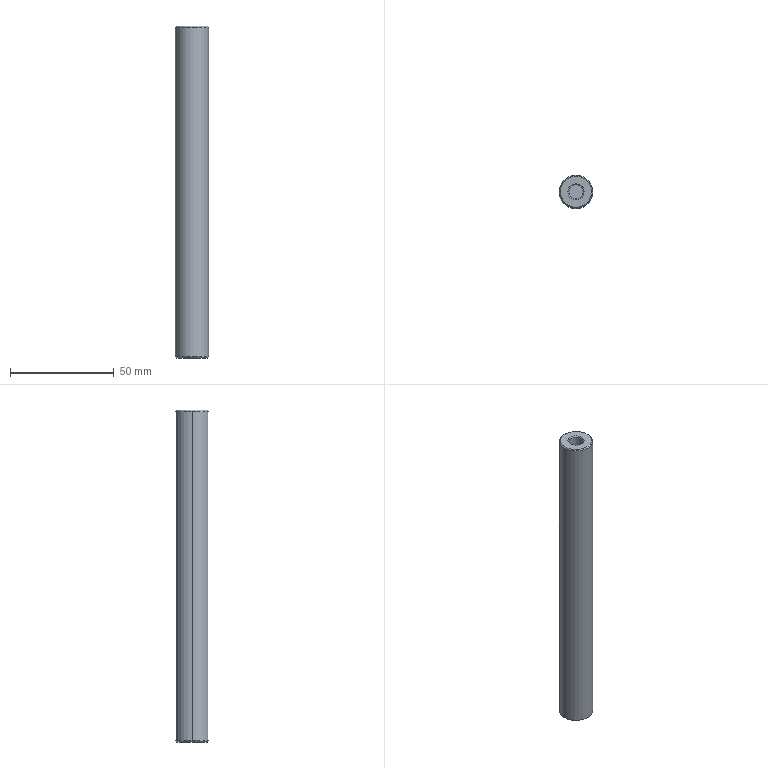Part | STEP file | Column | 1 solid | 18 faces | box 16 x 16 x 160 mm | volume 30717 mm3 | cone 8 | cylinder 6 | plane 4 | commonest cylinder face diameters 6.8 x4 16 x2
STEP:
#1=CARTESIAN_POINT('',(0.,0.,0.));
#2=DIRECTION('',(0.,0.,1.));
#3=DIRECTION('',(1.,0.,0.));
#4=AXIS2_PLACEMENT_3D('',#1,#2,#3);
#5=CARTESIAN_POINT('',(-8.,0.,159.5));
#6=VERTEX_POINT('',#5);
#7=CARTESIAN_POINT('',(8.,0.,159.5));
#8=VERTEX_POINT('',#7);
#9=CARTESIAN_POINT('',(0.,0.,159.5));
#10=DIRECTION('',(0.,0.,-1.));
#11=DIRECTION('',(-1.,0.,0.));
#12=AXIS2_PLACEMENT_3D('',#9,#10,#11);
#13=CIRCLE('',#12,8.);
#14=CARTESIAN_POINT('',(0.,0.,160.));
#15=DIRECTION('',(0.,0.,-1.));
#16=DIRECTION('',(-1.,0.,0.));
#17=AXIS2_PLACEMENT_3D('',#14,#15,#16);
#18=CYLINDRICAL_SURFACE('',#17,8.);
#19=CARTESIAN_POINT('',(0.,0.5));
#20=DIRECTION('',(1.,0.));
#21=VECTOR('',#20,1.);
#22=LINE('',#19,#21);
#23=(GEOMETRIC_REPRESENTATION_CONTEXT(2)PARAMETRIC_REPRESENTATION_CONTEXT()REPRESENTATION_CONTEXT('',''));
#24=DEFINITIONAL_REPRESENTATION('',(#22),#23);
#25=PCURVE('',#18,#24);
#26=CARTESIAN_POINT('',(0.,0.,159.5));
#27=DIRECTION('',(0.,0.,-1.));
#28=DIRECTION('',(-1.,0.,0.));
#29=AXIS2_PLACEMENT_3D('',#26,#27,#28);
#30=CONICAL_SURFACE('',#29,8.,0.7854);
#31=CARTESIAN_POINT('',(0.,0.));
#32=DIRECTION('',(1.,0.));
#33=VECTOR('',#32,1.);
#34=LINE('',#31,#33);
#35=(GEOMETRIC_REPRESENTATION_CONTEXT(2)PARAMETRIC_REPRESENTATION_CONTEXT()REPRESENTATION_CONTEXT('',''));
#36=DEFINITIONAL_REPRESENTATION('',(#34),#35);
#37=PCURVE('',#30,#36);
#38=SURFACE_CURVE('',#13,(#25,#37),.PCURVE_S1.);
#39=EDGE_CURVE('',#6,#8,#38,.T.);
#40=ORIENTED_EDGE('',*,*,#39,.T.);
#41=CARTESIAN_POINT('',(8.,0.,0.5));
#42=VERTEX_POINT('',#41);
#43=CARTESIAN_POINT('',(8.,0.,160.));
#44=DIRECTION('',(0.,0.,-1.));
#45=VECTOR('',#44,1.);
#46=LINE('',#43,#45);
#47=CARTESIAN_POINT('',(3.142,0.));
#48=DIRECTION('',(0.,1.));
#49=VECTOR('',#48,1.);
#50=LINE('',#47,#49);
#51=(GEOMETRIC_REPRESENTATION_CONTEXT(2)PARAMETRIC_REPRESENTATION_CONTEXT()REPRESENTATION_CONTEXT('',''));
#52=DEFINITIONAL_REPRESENTATION('',(#50),#51);
#53=PCURVE('',#18,#52);
#54=CARTESIAN_POINT('',(0.,0.,160.));
#55=DIRECTION('',(0.,0.,-1.));
#56=DIRECTION('',(-1.,0.,0.));
#57=AXIS2_PLACEMENT_3D('',#54,#55,#56);
#58=CYLINDRICAL_SURFACE('',#57,8.);
#59=CARTESIAN_POINT('',(3.142,0.));
#60=DIRECTION('',(0.,1.));
#61=VECTOR('',#60,1.);
#62=LINE('',#59,#61);
#63=(GEOMETRIC_REPRESENTATION_CONTEXT(2)PARAMETRIC_REPRESENTATION_CONTEXT()REPRESENTATION_CONTEXT('',''));
#64=DEFINITIONAL_REPRESENTATION('',(#62),#63);
#65=PCURVE('',#58,#64);
#66=SURFACE_CURVE('',#46,(#53,#65),.PCURVE_S1.);
#67=EDGE_CURVE('',#8,#42,#66,.T.);
#68=ORIENTED_EDGE('',*,*,#67,.T.);
#69=CARTESIAN_POINT('',(-8.,0.,0.5));
#70=VERTEX_POINT('',#69);
#71=CARTESIAN_POINT('',(0.,0.,0.5));
#72=DIRECTION('',(0.,0.,1.));
#73=DIRECTION('',(-1.,0.,0.));
#74=AXIS2_PLACEMENT_3D('',#71,#72,#73);
#75=CIRCLE('',#74,8.);
#76=CARTESIAN_POINT('',(6.283,159.5));
#77=DIRECTION('',(-1.,0.));
#78=VECTOR('',#77,1.);
#79=LINE('',#76,#78);
#80=(GEOMETRIC_REPRESENTATION_CONTEXT(2)PARAMETRIC_REPRESENTATION_CONTEXT()REPRESENTATION_CONTEXT('',''));
#81=DEFINITIONAL_REPRESENTATION('',(#79),#80);
#82=PCURVE('',#18,#81);
#83=CARTESIAN_POINT('',(0.,0.,0.5));
#84=DIRECTION('',(0.,0.,1.));
#85=DIRECTION('',(1.,0.,0.));
#86=AXIS2_PLACEMENT_3D('',#83,#84,#85);
#87=CONICAL_SURFACE('',#86,8.,0.7854);
#88=CARTESIAN_POINT('',(-3.142,0.));
#89=DIRECTION('',(1.,0.));
#90=VECTOR('',#89,1.);
#91=LINE('',#88,#90);
#92=(GEOMETRIC_REPRESENTATION_CONTEXT(2)PARAMETRIC_REPRESENTATION_CONTEXT()REPRESENTATION_CONTEXT('',''));
#93=DEFINITIONAL_REPRESENTATION('',(#91),#92);
#94=PCURVE('',#87,#93);
#95=SURFACE_CURVE('',#75,(#82,#94),.PCURVE_S1.);
#96=EDGE_CURVE('',#42,#70,#95,.T.);
#97=ORIENTED_EDGE('',*,*,#96,.T.);
#98=CARTESIAN_POINT('',(-8.,0.,160.));
#99=DIRECTION('',(0.,0.,-1.));
#100=VECTOR('',#99,1.);
#101=LINE('',#98,#100);
#102=CARTESIAN_POINT('',(0.,0.));
#103=DIRECTION('',(0.,1.));
#104=VECTOR('',#103,1.);
#105=LINE('',#102,#104);
#106=(GEOMETRIC_REPRESENTATION_CONTEXT(2)PARAMETRIC_REPRESENTATION_CONTEXT()REPRESENTATION_CONTEXT('',''));
#107=DEFINITIONAL_REPRESENTATION('',(#105),#106);
#108=PCURVE('',#18,#107);
#109=CARTESIAN_POINT('',(6.283,0.));
#110=DIRECTION('',(0.,1.));
#111=VECTOR('',#110,1.);
#112=LINE('',#109,#111);
#113=(GEOMETRIC_REPRESENTATION_CONTEXT(2)PARAMETRIC_REPRESENTATION_CONTEXT()REPRESENTATION_CONTEXT('',''));
#114=DEFINITIONAL_REPRESENTATION('',(#112),#113);
#115=PCURVE('',#58,#114);
#116=SURFACE_CURVE('',#101,(#108,#115),.PCURVE_S1.);
#117=EDGE_CURVE('',#6,#70,#116,.T.);
#118=ORIENTED_EDGE('',*,*,#117,.F.);
#119=EDGE_LOOP('',(#40,#68,#97,#118));
#120=FACE_BOUND('',#119,.T.);
#121=ADVANCED_FACE('',(#120),#18,.T.);
#122=CARTESIAN_POINT('',(7.5,0.,0.));
#123=VERTEX_POINT('',#122);
#124=CARTESIAN_POINT('',(-7.5,0.,0.));
#125=VERTEX_POINT('',#124);
#126=CARTESIAN_POINT('',(0.,0.,0.));
#127=DIRECTION('',(0.,0.,1.));
#128=DIRECTION('',(1.,0.,0.));
#129=AXIS2_PLACEMENT_3D('',#126,#127,#128);
#130=CIRCLE('',#129,7.5);
#131=CARTESIAN_POINT('',(0.,-0.5));
#132=DIRECTION('',(1.,0.));
#133=VECTOR('',#132,1.);
#134=LINE('',#131,#133);
#135=(GEOMETRIC_REPRESENTATION_CONTEXT(2)PARAMETRIC_REPRESENTATION_CONTEXT()REPRESENTATION_CONTEXT('',''));
#136=DEFINITIONAL_REPRESENTATION('',(#134),#135);
#137=PCURVE('',#87,#136);
#138=CARTESIAN_POINT('',(0.,0.,0.));
#139=DIRECTION('',(0.,0.,1.));
#140=DIRECTION('',(1.,0.,0.));
#141=AXIS2_PLACEMENT_3D('',#138,#139,#140);
#142=PLANE('',#141);
#143=CARTESIAN_POINT('',(0.,0.));
#144=DIRECTION('',(1.,0.));
#145=AXIS2_PLACEMENT_2D('',#143,#144);
#146=CIRCLE('',#145,7.5);
#147=(GEOMETRIC_REPRESENTATION_CONTEXT(2)PARAMETRIC_REPRESENTATION_CONTEXT()REPRESENTATION_CONTEXT('',''));
#148=DEFINITIONAL_REPRESENTATION('',(#146),#147);
#149=PCURVE('',#142,#148);
#150=SURFACE_CURVE('',#130,(#137,#149),.PCURVE_S1.);
#151=EDGE_CURVE('',#123,#125,#150,.T.);
#152=ORIENTED_EDGE('',*,*,#151,.T.);
#153=CARTESIAN_POINT('',(-8.,0.,0.5));
#154=DIRECTION('',(-0.7071,0.,0.7071));
#155=VECTOR('',#154,1.);
#156=LINE('',#153,#155);
#157=CARTESIAN_POINT('',(3.142,0.));
#158=DIRECTION('',(0.,1.));
#159=VECTOR('',#158,1.);
#160=LINE('',#157,#159);
#161=(GEOMETRIC_REPRESENTATION_CONTEXT(2)PARAMETRIC_REPRESENTATION_CONTEXT()REPRESENTATION_CONTEXT('',''));
#162=DEFINITIONAL_REPRESENTATION('',(#160),#161);
#163=PCURVE('',#87,#162);
#164=CARTESIAN_POINT('',(0.,0.,0.5));
#165=DIRECTION('',(0.,0.,1.));
#166=DIRECTION('',(1.,0.,0.));
#167=AXIS2_PLACEMENT_3D('',#164,#165,#166);
#168=CONICAL_SURFACE('',#167,8.,0.7854);
#169=CARTESIAN_POINT('',(3.142,0.));
#170=DIRECTION('',(0.,1.));
#171=VECTOR('',#170,1.);
#172=LINE('',#169,#171);
#173=(GEOMETRIC_REPRESENTATION_CONTEXT(2)PARAMETRIC_REPRESENTATION_CONTEXT()REPRESENTATION_CONTEXT('',''));
#174=DEFINITIONAL_REPRESENTATION('',(#172),#173);
#175=PCURVE('',#168,#174);
#176=SURFACE_CURVE('',#156,(#163,#175),.PCURVE_S1.);
#177=EDGE_CURVE('',#125,#70,#176,.T.);
#178=ORIENTED_EDGE('',*,*,#177,.T.);
#179=ORIENTED_EDGE('',*,*,#96,.F.);
#180=CARTESIAN_POINT('',(8.,0.,0.5));
#181=DIRECTION('',(0.7071,0.,0.7071));
#182=VECTOR('',#181,1.);
#183=LINE('',#180,#182);
#184=CARTESIAN_POINT('',(0.,0.));
#185=DIRECTION('',(0.,1.));
#186=VECTOR('',#185,1.);
#187=LINE('',#184,#186);
#188=(GEOMETRIC_REPRESENTATION_CONTEXT(2)PARAMETRIC_REPRESENTATION_CONTEXT()REPRESENTATION_CONTEXT('',''));
#189=DEFINITIONAL_REPRESENTATION('',(#187),#188);
#190=PCURVE('',#87,#189);
#191=CARTESIAN_POINT('',(6.283,0.));
#192=DIRECTION('',(0.,1.));
#193=VECTOR('',#192,1.);
#194=LINE('',#191,#193);
#195=(GEOMETRIC_REPRESENTATION_CONTEXT(2)PARAMETRIC_REPRESENTATION_CONTEXT()REPRESENTATION_CONTEXT('',''));
#196=DEFINITIONAL_REPRESENTATION('',(#194),#195);
#197=PCURVE('',#168,#196);
#198=SURFACE_CURVE('',#183,(#190,#197),.PCURVE_S1.);
#199=EDGE_CURVE('',#123,#42,#198,.T.);
#200=ORIENTED_EDGE('',*,*,#199,.F.);
#201=EDGE_LOOP('',(#152,#178,#179,#200));
#202=FACE_BOUND('',#201,.T.);
#203=ADVANCED_FACE('',(#202),#87,.T.);
#204=CARTESIAN_POINT('',(-7.5,0.,160.));
#205=VERTEX_POINT('',#204);
#206=CARTESIAN_POINT('',(7.5,0.,160.));
#207=VERTEX_POINT('',#206);
#208=CARTESIAN_POINT('',(0.,0.,160.));
#209=DIRECTION('',(0.,0.,-1.));
#210=DIRECTION('',(-1.,0.,0.));
#211=AXIS2_PLACEMENT_3D('',#208,#209,#210);
#212=CIRCLE('',#211,7.5);
#213=CARTESIAN_POINT('',(0.,-0.5));
#214=DIRECTION('',(1.,0.));
#215=VECTOR('',#214,1.);
#216=LINE('',#213,#215);
#217=(GEOMETRIC_REPRESENTATION_CONTEXT(2)PARAMETRIC_REPRESENTATION_CONTEXT()REPRESENTATION_CONTEXT('',''));
#218=DEFINITIONAL_REPRESENTATION('',(#216),#217);
#219=PCURVE('',#30,#218);
#220=CARTESIAN_POINT('',(0.,0.,160.));
#221=DIRECTION('',(0.,0.,1.));
#222=DIRECTION('',(1.,0.,0.));
#223=AXIS2_PLACEMENT_3D('',#220,#221,#222);
#224=PLANE('',#223);
#225=CARTESIAN_POINT('',(-7.5,0.));
#226=CARTESIAN_POINT('',(-7.5,12.99));
#227=CARTESIAN_POINT('',(3.75,6.495));
#228=CARTESIAN_POINT('',(15.,0.));
#229=CARTESIAN_POINT('',(3.75,-6.495));
#230=CARTESIAN_POINT('',(-7.5,-12.99));
#231=CARTESIAN_POINT('',(-7.5,0.));
#232=(BOUNDED_CURVE()B_SPLINE_CURVE(2,(#225,#226,#227,#228,#229,#230,#231),.UNSPECIFIED.,.T.,.F.)B_SPLINE_CURVE_WITH_KNOTS((1,2,2,2,2,1),(-2.094,0.,2.094,4.189,6.283,8.378),.UNSPECIFIED.)CURVE()GEOMETRIC_REPRESENTATION_ITEM()RATIONAL_B_SPLINE_CURVE((1.,0.5,1.,0.5,1.,0.5,1.))REPRESENTATION_ITEM(''));
#233=(GEOMETRIC_REPRESENTATION_CONTEXT(2)PARAMETRIC_REPRESENTATION_CONTEXT()REPRESENTATION_CONTEXT('',''));
#234=DEFINITIONAL_REPRESENTATION('',(#232),#233);
#235=PCURVE('',#224,#234);
#236=SURFACE_CURVE('',#212,(#219,#235),.PCURVE_S1.);
#237=EDGE_CURVE('',#205,#207,#236,.T.);
#238=ORIENTED_EDGE('',*,*,#237,.T.);
#239=CARTESIAN_POINT('',(8.,0.,159.5));
#240=DIRECTION('',(0.7071,0.,-0.7071));
#241=VECTOR('',#240,1.);
#242=LINE('',#239,#241);
#243=CARTESIAN_POINT('',(3.142,0.));
#244=DIRECTION('',(0.,1.));
#245=VECTOR('',#244,1.);
#246=LINE('',#243,#245);
#247=(GEOMETRIC_REPRESENTATION_CONTEXT(2)PARAMETRIC_REPRESENTATION_CONTEXT()REPRESENTATION_CONTEXT('',''));
#248=DEFINITIONAL_REPRESENTATION('',(#246),#247);
#249=PCURVE('',#30,#248);
#250=CARTESIAN_POINT('',(0.,0.,159.5));
#251=DIRECTION('',(0.,0.,-1.));
#252=DIRECTION('',(-1.,0.,0.));
#253=AXIS2_PLACEMENT_3D('',#250,#251,#252);
#254=CONICAL_SURFACE('',#253,8.,0.7854);
#255=CARTESIAN_POINT('',(3.142,0.));
#256=DIRECTION('',(0.,1.));
#257=VECTOR('',#256,1.);
#258=LINE('',#255,#257);
#259=(GEOMETRIC_REPRESENTATION_CONTEXT(2)PARAMETRIC_REPRESENTATION_CONTEXT()REPRESENTATION_CONTEXT('',''));
#260=DEFINITIONAL_REPRESENTATION('',(#258),#259);
#261=PCURVE('',#254,#260);
#262=SURFACE_CURVE('',#242,(#249,#261),.PCURVE_S1.);
#263=EDGE_CURVE('',#207,#8,#262,.T.);
#264=ORIENTED_EDGE('',*,*,#263,.T.);
#265=ORIENTED_EDGE('',*,*,#39,.F.);
#266=CARTESIAN_POINT('',(-8.,0.,159.5));
#267=DIRECTION('',(-0.7071,0.,-0.7071));
#268=VECTOR('',#267,1.);
#269=LINE('',#266,#268);
#270=CARTESIAN_POINT('',(0.,0.));
#271=DIRECTION('',(0.,1.));
#272=VECTOR('',#271,1.);
#273=LINE('',#270,#272);
#274=(GEOMETRIC_REPRESENTATION_CONTEXT(2)PARAMETRIC_REPRESENTATION_CONTEXT()REPRESENTATION_CONTEXT('',''));
#275=DEFINITIONAL_REPRESENTATION('',(#273),#274);
#276=PCURVE('',#30,#275);
#277=CARTESIAN_POINT('',(6.283,0.));
#278=DIRECTION('',(0.,1.));
#279=VECTOR('',#278,1.);
#280=LINE('',#277,#279);
#281=(GEOMETRIC_REPRESENTATION_CONTEXT(2)PARAMETRIC_REPRESENTATION_CONTEXT()REPRESENTATION_CONTEXT('',''));
#282=DEFINITIONAL_REPRESENTATION('',(#280),#281);
#283=PCURVE('',#254,#282);
#284=SURFACE_CURVE('',#269,(#276,#283),.PCURVE_S1.);
#285=EDGE_CURVE('',#205,#6,#284,.T.);
#286=ORIENTED_EDGE('',*,*,#285,.F.);
#287=EDGE_LOOP('',(#238,#264,#265,#286));
#288=FACE_BOUND('',#287,.T.);
#289=ADVANCED_FACE('',(#288),#30,.T.);
#290=CARTESIAN_POINT('',(-3.4,0.,0.5));
#291=VERTEX_POINT('',#290);
#292=CARTESIAN_POINT('',(-3.9,0.,0.));
#293=VERTEX_POINT('',#292);
#294=CARTESIAN_POINT('',(-3.9,0.,0.));
#295=DIRECTION('',(-0.7071,0.,-0.7071));
#296=VECTOR('',#295,1.);
#297=LINE('',#294,#296);
#298=CARTESIAN_POINT('',(0.,0.,0.));
#299=DIRECTION('',(0.,0.,-1.));
#300=DIRECTION('',(-1.,0.,0.));
#301=AXIS2_PLACEMENT_3D('',#298,#299,#300);
#302=CONICAL_SURFACE('',#301,3.9,0.7854);
#303=CARTESIAN_POINT('',(6.283,0.));
#304=DIRECTION('',(0.,1.));
#305=VECTOR('',#304,1.);
#306=LINE('',#303,#305);
#307=(GEOMETRIC_REPRESENTATION_CONTEXT(2)PARAMETRIC_REPRESENTATION_CONTEXT()REPRESENTATION_CONTEXT('',''));
#308=DEFINITIONAL_REPRESENTATION('',(#306),#307);
#309=PCURVE('',#302,#308);
#310=CARTESIAN_POINT('',(0.,0.,0.));
#311=DIRECTION('',(0.,0.,-1.));
#312=DIRECTION('',(-1.,0.,0.));
#313=AXIS2_PLACEMENT_3D('',#310,#311,#312);
#314=CONICAL_SURFACE('',#313,3.9,0.7854);
#315=CARTESIAN_POINT('',(0.,0.));
#316=DIRECTION('',(0.,1.));
#317=VECTOR('',#316,1.);
#318=LINE('',#315,#317);
#319=(GEOMETRIC_REPRESENTATION_CONTEXT(2)PARAMETRIC_REPRESENTATION_CONTEXT()REPRESENTATION_CONTEXT('',''));
#320=DEFINITIONAL_REPRESENTATION('',(#318),#319);
#321=PCURVE('',#314,#320);
#322=SURFACE_CURVE('',#297,(#309,#321),.PCURVE_S1.);
#323=EDGE_CURVE('',#291,#293,#322,.T.);
#324=ORIENTED_EDGE('',*,*,#323,.T.);
#325=CARTESIAN_POINT('',(3.9,0.,0.));
#326=VERTEX_POINT('',#325);
#327=CARTESIAN_POINT('',(0.,0.,0.));
#328=DIRECTION('',(0.,0.,-1.));
#329=DIRECTION('',(-1.,0.,0.));
#330=AXIS2_PLACEMENT_3D('',#327,#328,#329);
#331=CIRCLE('',#330,3.9);
#332=CARTESIAN_POINT('',(0.,0.));
#333=DIRECTION('',(1.,0.));
#334=VECTOR('',#333,1.);
#335=LINE('',#332,#334);
#336=(GEOMETRIC_REPRESENTATION_CONTEXT(2)PARAMETRIC_REPRESENTATION_CONTEXT()REPRESENTATION_CONTEXT('',''));
#337=DEFINITIONAL_REPRESENTATION('',(#335),#336);
#338=PCURVE('',#302,#337);
#339=CARTESIAN_POINT('',(-3.9,0.));
#340=CARTESIAN_POINT('',(-3.9,6.755));
#341=CARTESIAN_POINT('',(1.95,3.377));
#342=CARTESIAN_POINT('',(7.8,0.));
#343=CARTESIAN_POINT('',(1.95,-3.377));
#344=CARTESIAN_POINT('',(-3.9,-6.755));
#345=CARTESIAN_POINT('',(-3.9,0.));
#346=(BOUNDED_CURVE()B_SPLINE_CURVE(2,(#339,#340,#341,#342,#343,#344,#345),.UNSPECIFIED.,.T.,.F.)B_SPLINE_CURVE_WITH_KNOTS((1,2,2,2,2,1),(-2.094,0.,2.094,4.189,6.283,8.378),.UNSPECIFIED.)CURVE()GEOMETRIC_REPRESENTATION_ITEM()RATIONAL_B_SPLINE_CURVE((1.,0.5,1.,0.5,1.,0.5,1.))REPRESENTATION_ITEM(''));
#347=(GEOMETRIC_REPRESENTATION_CONTEXT(2)PARAMETRIC_REPRESENTATION_CONTEXT()REPRESENTATION_CONTEXT('',''));
#348=DEFINITIONAL_REPRESENTATION('',(#346),#347);
#349=PCURVE('',#142,#348);
#350=SURFACE_CURVE('',#331,(#338,#349),.PCURVE_S1.);
#351=EDGE_CURVE('',#326,#293,#350,.T.);
#352=ORIENTED_EDGE('',*,*,#351,.F.);
#353=CARTESIAN_POINT('',(3.4,0.,0.5));
#354=VERTEX_POINT('',#353);
#355=CARTESIAN_POINT('',(3.9,0.,0.));
#356=DIRECTION('',(0.7071,0.,-0.7071));
#357=VECTOR('',#356,1.);
#358=LINE('',#355,#357);
#359=CARTESIAN_POINT('',(3.142,0.));
#360=DIRECTION('',(0.,1.));
#361=VECTOR('',#360,1.);
#362=LINE('',#359,#361);
#363=(GEOMETRIC_REPRESENTATION_CONTEXT(2)PARAMETRIC_REPRESENTATION_CONTEXT()REPRESENTATION_CONTEXT('',''));
#364=DEFINITIONAL_REPRESENTATION('',(#362),#363);
#365=PCURVE('',#302,#364);
#366=CARTESIAN_POINT('',(3.142,0.));
#367=DIRECTION('',(0.,1.));
#368=VECTOR('',#367,1.);
#369=LINE('',#366,#368);
#370=(GEOMETRIC_REPRESENTATION_CONTEXT(2)PARAMETRIC_REPRESENTATION_CONTEXT()REPRESENTATION_CONTEXT('',''));
#371=DEFINITIONAL_REPRESENTATION('',(#369),#370);
#372=PCURVE('',#314,#371);
#373=SURFACE_CURVE('',#358,(#365,#372),.PCURVE_S1.);
#374=EDGE_CURVE('',#354,#326,#373,.T.);
#375=ORIENTED_EDGE('',*,*,#374,.F.);
#376=CARTESIAN_POINT('',(0.,0.,0.5));
#377=DIRECTION('',(0.,0.,-1.));
#378=DIRECTION('',(-1.,0.,0.));
#379=AXIS2_PLACEMENT_3D('',#376,#377,#378);
#380=CIRCLE('',#379,3.4);
#381=CARTESIAN_POINT('',(0.,-0.5));
#382=DIRECTION('',(1.,0.));
#383=VECTOR('',#382,1.);
#384=LINE('',#381,#383);
#385=(GEOMETRIC_REPRESENTATION_CONTEXT(2)PARAMETRIC_REPRESENTATION_CONTEXT()REPRESENTATION_CONTEXT('',''));
#386=DEFINITIONAL_REPRESENTATION('',(#384),#385);
#387=PCURVE('',#302,#386);
#388=CARTESIAN_POINT('',(0.,0.,0.));
#389=DIRECTION('',(0.,0.,-1.));
#390=DIRECTION('',(-1.,0.,0.));
#391=AXIS2_PLACEMENT_3D('',#388,#389,#390);
#392=CYLINDRICAL_SURFACE('',#391,3.4);
#393=CARTESIAN_POINT('',(0.,-0.5));
#394=DIRECTION('',(1.,0.));
#395=VECTOR('',#394,1.);
#396=LINE('',#393,#395);
#397=(GEOMETRIC_REPRESENTATION_CONTEXT(2)PARAMETRIC_REPRESENTATION_CONTEXT()REPRESENTATION_CONTEXT('',''));
#398=DEFINITIONAL_REPRESENTATION('',(#396),#397);
#399=PCURVE('',#392,#398);
#400=SURFACE_CURVE('',#380,(#387,#399),.PCURVE_S1.);
#401=EDGE_CURVE('',#354,#291,#400,.T.);
#402=ORIENTED_EDGE('',*,*,#401,.T.);
#403=EDGE_LOOP('',(#324,#352,#375,#402));
#404=FACE_BOUND('',#403,.F.);
#405=ADVANCED_FACE('',(#404),#302,.F.);
#406=CARTESIAN_POINT('',(3.4,0.,159.5));
#407=VERTEX_POINT('',#406);
#408=CARTESIAN_POINT('',(3.9,0.,160.));
#409=VERTEX_POINT('',#408);
#410=CARTESIAN_POINT('',(3.9,0.,160.));
#411=DIRECTION('',(0.7071,0.,0.7071));
#412=VECTOR('',#411,1.);
#413=LINE('',#410,#412);
#414=CARTESIAN_POINT('',(0.,0.,160.));
#415=DIRECTION('',(0.,0.,1.));
#416=DIRECTION('',(1.,0.,0.));
#417=AXIS2_PLACEMENT_3D('',#414,#415,#416);
#418=CONICAL_SURFACE('',#417,3.9,0.7854);
#419=CARTESIAN_POINT('',(6.283,0.));
#420=DIRECTION('',(0.,1.));
#421=VECTOR('',#420,1.);
#422=LINE('',#419,#421);
#423=(GEOMETRIC_REPRESENTATION_CONTEXT(2)PARAMETRIC_REPRESENTATION_CONTEXT()REPRESENTATION_CONTEXT('',''));
#424=DEFINITIONAL_REPRESENTATION('',(#422),#423);
#425=PCURVE('',#418,#424);
#426=CARTESIAN_POINT('',(0.,0.,160.));
#427=DIRECTION('',(0.,0.,1.));
#428=DIRECTION('',(1.,0.,0.));
#429=AXIS2_PLACEMENT_3D('',#426,#427,#428);
#430=CONICAL_SURFACE('',#429,3.9,0.7854);
#431=CARTESIAN_POINT('',(0.,0.));
#432=DIRECTION('',(0.,1.));
#433=VECTOR('',#432,1.);
#434=LINE('',#431,#433);
#435=(GEOMETRIC_REPRESENTATION_CONTEXT(2)PARAMETRIC_REPRESENTATION_CONTEXT()REPRESENTATION_CONTEXT('',''));
#436=DEFINITIONAL_REPRESENTATION('',(#434),#435);
#437=PCURVE('',#430,#436);
#438=SURFACE_CURVE('',#413,(#425,#437),.PCURVE_S1.);
#439=EDGE_CURVE('',#407,#409,#438,.T.);
#440=ORIENTED_EDGE('',*,*,#439,.T.);
#441=CARTESIAN_POINT('',(-3.9,0.,160.));
#442=VERTEX_POINT('',#441);
#443=CARTESIAN_POINT('',(0.,0.,160.));
#444=DIRECTION('',(0.,0.,-1.));
#445=DIRECTION('',(1.,0.,0.));
#446=AXIS2_PLACEMENT_3D('',#443,#444,#445);
#447=CIRCLE('',#446,3.9);
#448=CARTESIAN_POINT('',(6.283,0.));
#449=DIRECTION('',(-1.,0.));
#450=VECTOR('',#449,1.);
#451=LINE('',#448,#450);
#452=(GEOMETRIC_REPRESENTATION_CONTEXT(2)PARAMETRIC_REPRESENTATION_CONTEXT()REPRESENTATION_CONTEXT('',''));
#453=DEFINITIONAL_REPRESENTATION('',(#451),#452);
#454=PCURVE('',#418,#453);
#455=CARTESIAN_POINT('',(3.9,0.));
#456=CARTESIAN_POINT('',(3.9,-6.755));
#457=CARTESIAN_POINT('',(-1.95,-3.377));
#458=CARTESIAN_POINT('',(-7.8,0.));
#459=CARTESIAN_POINT('',(-1.95,3.377));
#460=CARTESIAN_POINT('',(3.9,6.755));
#461=CARTESIAN_POINT('',(3.9,0.));
#462=(BOUNDED_CURVE()B_SPLINE_CURVE(2,(#455,#456,#457,#458,#459,#460,#461),.UNSPECIFIED.,.T.,.F.)B_SPLINE_CURVE_WITH_KNOTS((1,2,2,2,2,1),(-2.094,0.,2.094,4.189,6.283,8.378),.UNSPECIFIED.)CURVE()GEOMETRIC_REPRESENTATION_ITEM()RATIONAL_B_SPLINE_CURVE((1.,0.5,1.,0.5,1.,0.5,1.))REPRESENTATION_ITEM(''));
#463=(GEOMETRIC_REPRESENTATION_CONTEXT(2)PARAMETRIC_REPRESENTATION_CONTEXT()REPRESENTATION_CONTEXT('',''));
#464=DEFINITIONAL_REPRESENTATION('',(#462),#463);
#465=PCURVE('',#224,#464);
#466=SURFACE_CURVE('',#447,(#454,#465),.PCURVE_S1.);
#467=EDGE_CURVE('',#409,#442,#466,.T.);
#468=ORIENTED_EDGE('',*,*,#467,.T.);
#469=CARTESIAN_POINT('',(-3.4,0.,159.5));
#470=VERTEX_POINT('',#469);
#471=CARTESIAN_POINT('',(-3.9,0.,160.));
#472=DIRECTION('',(-0.7071,0.,0.7071));
#473=VECTOR('',#472,1.);
#474=LINE('',#471,#473);
#475=CARTESIAN_POINT('',(3.142,0.));
#476=DIRECTION('',(0.,1.));
#477=VECTOR('',#476,1.);
#478=LINE('',#475,#477);
#479=(GEOMETRIC_REPRESENTATION_CONTEXT(2)PARAMETRIC_REPRESENTATION_CONTEXT()REPRESENTATION_CONTEXT('',''));
#480=DEFINITIONAL_REPRESENTATION('',(#478),#479);
#481=PCURVE('',#418,#480);
#482=CARTESIAN_POINT('',(3.142,0.));
#483=DIRECTION('',(0.,1.));
#484=VECTOR('',#483,1.);
#485=LINE('',#482,#484);
#486=(GEOMETRIC_REPRESENTATION_CONTEXT(2)PARAMETRIC_REPRESENTATION_CONTEXT()REPRESENTATION_CONTEXT('',''));
#487=DEFINITIONAL_REPRESENTATION('',(#485),#486);
#488=PCURVE('',#430,#487);
#489=SURFACE_CURVE('',#474,(#481,#488),.PCURVE_S1.);
#490=EDGE_CURVE('',#470,#442,#489,.T.);
#491=ORIENTED_EDGE('',*,*,#490,.F.);
#492=CARTESIAN_POINT('',(0.,0.,159.5));
#493=DIRECTION('',(0.,0.,1.));
#494=DIRECTION('',(1.,0.,0.));
#495=AXIS2_PLACEMENT_3D('',#492,#493,#494);
#496=CIRCLE('',#495,3.4);
#497=CARTESIAN_POINT('',(0.,-0.5));
#498=DIRECTION('',(1.,0.));
#499=VECTOR('',#498,1.);
#500=LINE('',#497,#499);
#501=(GEOMETRIC_REPRESENTATION_CONTEXT(2)PARAMETRIC_REPRESENTATION_CONTEXT()REPRESENTATION_CONTEXT('',''));
#502=DEFINITIONAL_REPRESENTATION('',(#500),#501);
#503=PCURVE('',#418,#502);
#504=CARTESIAN_POINT('',(0.,0.,160.));
#505=DIRECTION('',(0.,0.,1.));
#506=DIRECTION('',(1.,0.,0.));
#507=AXIS2_PLACEMENT_3D('',#504,#505,#506);
#508=CYLINDRICAL_SURFACE('',#507,3.4);
#509=CARTESIAN_POINT('',(0.,-0.5));
#510=DIRECTION('',(1.,0.));
#511=VECTOR('',#510,1.);
#512=LINE('',#509,#511);
#513=(GEOMETRIC_REPRESENTATION_CONTEXT(2)PARAMETRIC_REPRESENTATION_CONTEXT()REPRESENTATION_CONTEXT('',''));
#514=DEFINITIONAL_REPRESENTATION('',(#512),#513);
#515=PCURVE('',#508,#514);
#516=SURFACE_CURVE('',#496,(#503,#515),.PCURVE_S1.);
#517=EDGE_CURVE('',#470,#407,#516,.T.);
#518=ORIENTED_EDGE('',*,*,#517,.T.);
#519=EDGE_LOOP('',(#440,#468,#491,#518));
#520=FACE_BOUND('',#519,.F.);
#521=ADVANCED_FACE('',(#520),#418,.F.);
#522=CARTESIAN_POINT('',(-3.4,0.,19.75));
#523=VERTEX_POINT('',#522);
#524=CARTESIAN_POINT('',(-3.4,0.,0.));
#525=DIRECTION('',(0.,0.,-1.));
#526=VECTOR('',#525,1.);
#527=LINE('',#524,#526);
#528=CARTESIAN_POINT('',(6.283,0.));
#529=DIRECTION('',(0.,1.));
#530=VECTOR('',#529,1.);
#531=LINE('',#528,#530);
#532=(GEOMETRIC_REPRESENTATION_CONTEXT(2)PARAMETRIC_REPRESENTATION_CONTEXT()REPRESENTATION_CONTEXT('',''));
#533=DEFINITIONAL_REPRESENTATION('',(#531),#532);
#534=PCURVE('',#392,#533);
#535=CARTESIAN_POINT('',(0.,0.,0.));
#536=DIRECTION('',(0.,0.,-1.));
#537=DIRECTION('',(-1.,0.,0.));
#538=AXIS2_PLACEMENT_3D('',#535,#536,#537);
#539=CYLINDRICAL_SURFACE('',#538,3.4);
#540=CARTESIAN_POINT('',(0.,0.));
#541=DIRECTION('',(0.,1.));
#542=VECTOR('',#541,1.);
#543=LINE('',#540,#542);
#544=(GEOMETRIC_REPRESENTATION_CONTEXT(2)PARAMETRIC_REPRESENTATION_CONTEXT()REPRESENTATION_CONTEXT('',''));
#545=DEFINITIONAL_REPRESENTATION('',(#543),#544);
#546=PCURVE('',#539,#545);
#547=SURFACE_CURVE('',#527,(#534,#546),.PCURVE_S1.);
#548=EDGE_CURVE('',#523,#291,#547,.T.);
#549=ORIENTED_EDGE('',*,*,#548,.T.);
#550=ORIENTED_EDGE('',*,*,#401,.F.);
#551=CARTESIAN_POINT('',(3.4,0.,19.75));
#552=VERTEX_POINT('',#551);
#553=CARTESIAN_POINT('',(3.4,0.,0.));
#554=DIRECTION('',(0.,0.,-1.));
#555=VECTOR('',#554,1.);
#556=LINE('',#553,#555);
#557=CARTESIAN_POINT('',(3.142,0.));
#558=DIRECTION('',(0.,1.));
#559=VECTOR('',#558,1.);
#560=LINE('',#557,#559);
#561=(GEOMETRIC_REPRESENTATION_CONTEXT(2)PARAMETRIC_REPRESENTATION_CONTEXT()REPRESENTATION_CONTEXT('',''));
#562=DEFINITIONAL_REPRESENTATION('',(#560),#561);
#563=PCURVE('',#392,#562);
#564=CARTESIAN_POINT('',(3.142,0.));
#565=DIRECTION('',(0.,1.));
#566=VECTOR('',#565,1.);
#567=LINE('',#564,#566);
#568=(GEOMETRIC_REPRESENTATION_CONTEXT(2)PARAMETRIC_REPRESENTATION_CONTEXT()REPRESENTATION_CONTEXT('',''));
#569=DEFINITIONAL_REPRESENTATION('',(#567),#568);
#570=PCURVE('',#539,#569);
#571=SURFACE_CURVE('',#556,(#563,#570),.PCURVE_S1.);
#572=EDGE_CURVE('',#552,#354,#571,.T.);
#573=ORIENTED_EDGE('',*,*,#572,.F.);
#574=CARTESIAN_POINT('',(0.,0.,19.75));
#575=DIRECTION('',(0.,0.,-1.));
#576=DIRECTION('',(-1.,0.,0.));
#577=AXIS2_PLACEMENT_3D('',#574,#575,#576);
#578=CIRCLE('',#577,3.4);
#579=CARTESIAN_POINT('',(0.,-19.75));
#580=DIRECTION('',(1.,0.));
#581=VECTOR('',#580,1.);
#582=LINE('',#579,#581);
#583=(GEOMETRIC_REPRESENTATION_CONTEXT(2)PARAMETRIC_REPRESENTATION_CONTEXT()REPRESENTATION_CONTEXT('',''));
#584=DEFINITIONAL_REPRESENTATION('',(#582),#583);
#585=PCURVE('',#392,#584);
#586=CARTESIAN_POINT('',(0.,0.,19.75));
#587=DIRECTION('',(0.,0.,1.));
#588=DIRECTION('',(1.,0.,0.));
#589=AXIS2_PLACEMENT_3D('',#586,#587,#588);
#590=PLANE('',#589);
#591=CARTESIAN_POINT('',(-3.4,0.));
#592=CARTESIAN_POINT('',(-3.4,5.889));
#593=CARTESIAN_POINT('',(1.7,2.944));
#594=CARTESIAN_POINT('',(6.8,0.));
#595=CARTESIAN_POINT('',(1.7,-2.944));
#596=CARTESIAN_POINT('',(-3.4,-5.889));
#597=CARTESIAN_POINT('',(-3.4,0.));
#598=(BOUNDED_CURVE()B_SPLINE_CURVE(2,(#591,#592,#593,#594,#595,#596,#597),.UNSPECIFIED.,.T.,.F.)B_SPLINE_CURVE_WITH_KNOTS((1,2,2,2,2,1),(-2.094,0.,2.094,4.189,6.283,8.378),.UNSPECIFIED.)CURVE()GEOMETRIC_REPRESENTATION_ITEM()RATIONAL_B_SPLINE_CURVE((1.,0.5,1.,0.5,1.,0.5,1.))REPRESENTATION_ITEM(''));
#599=(GEOMETRIC_REPRESENTATION_CONTEXT(2)PARAMETRIC_REPRESENTATION_CONTEXT()REPRESENTATION_CONTEXT('',''));
#600=DEFINITIONAL_REPRESENTATION('',(#598),#599);
#601=PCURVE('',#590,#600);
#602=SURFACE_CURVE('',#578,(#585,#601),.PCURVE_S1.);
#603=EDGE_CURVE('',#552,#523,#602,.T.);
#604=ORIENTED_EDGE('',*,*,#603,.T.);
#605=EDGE_LOOP('',(#549,#550,#573,#604));
#606=FACE_BOUND('',#605,.F.);
#607=ADVANCED_FACE('',(#606),#392,.F.);
#608=CARTESIAN_POINT('',(3.4,0.,140.25));
#609=VERTEX_POINT('',#608);
#610=CARTESIAN_POINT('',(3.4,0.,160.));
#611=DIRECTION('',(0.,0.,1.));
#612=VECTOR('',#611,1.);
#613=LINE('',#610,#612);
#614=CARTESIAN_POINT('',(6.283,0.));
#615=DIRECTION('',(0.,1.));
#616=VECTOR('',#615,1.);
#617=LINE('',#614,#616);
#618=(GEOMETRIC_REPRESENTATION_CONTEXT(2)PARAMETRIC_REPRESENTATION_CONTEXT()REPRESENTATION_CONTEXT('',''));
#619=DEFINITIONAL_REPRESENTATION('',(#617),#618);
#620=PCURVE('',#508,#619);
#621=CARTESIAN_POINT('',(0.,0.,160.));
#622=DIRECTION('',(0.,0.,1.));
#623=DIRECTION('',(1.,0.,0.));
#624=AXIS2_PLACEMENT_3D('',#621,#622,#623);
#625=CYLINDRICAL_SURFACE('',#624,3.4);
#626=CARTESIAN_POINT('',(0.,0.));
#627=DIRECTION('',(0.,1.));
#628=VECTOR('',#627,1.);
#629=LINE('',#626,#628);
#630=(GEOMETRIC_REPRESENTATION_CONTEXT(2)PARAMETRIC_REPRESENTATION_CONTEXT()REPRESENTATION_CONTEXT('',''));
#631=DEFINITIONAL_REPRESENTATION('',(#629),#630);
#632=PCURVE('',#625,#631);
#633=SURFACE_CURVE('',#613,(#620,#632),.PCURVE_S1.);
#634=EDGE_CURVE('',#609,#407,#633,.T.);
#635=ORIENTED_EDGE('',*,*,#634,.T.);
#636=ORIENTED_EDGE('',*,*,#517,.F.);
#637=CARTESIAN_POINT('',(-3.4,0.,140.25));
#638=VERTEX_POINT('',#637);
#639=CARTESIAN_POINT('',(-3.4,0.,160.));
#640=DIRECTION('',(0.,0.,1.));
#641=VECTOR('',#640,1.);
#642=LINE('',#639,#641);
#643=CARTESIAN_POINT('',(3.142,0.));
#644=DIRECTION('',(0.,1.));
#645=VECTOR('',#644,1.);
#646=LINE('',#643,#645);
#647=(GEOMETRIC_REPRESENTATION_CONTEXT(2)PARAMETRIC_REPRESENTATION_CONTEXT()REPRESENTATION_CONTEXT('',''));
#648=DEFINITIONAL_REPRESENTATION('',(#646),#647);
#649=PCURVE('',#508,#648);
#650=CARTESIAN_POINT('',(3.142,0.));
#651=DIRECTION('',(0.,1.));
#652=VECTOR('',#651,1.);
#653=LINE('',#650,#652);
#654=(GEOMETRIC_REPRESENTATION_CONTEXT(2)PARAMETRIC_REPRESENTATION_CONTEXT()REPRESENTATION_CONTEXT('',''));
#655=DEFINITIONAL_REPRESENTATION('',(#653),#654);
#656=PCURVE('',#625,#655);
#657=SURFACE_CURVE('',#642,(#649,#656),.PCURVE_S1.);
#658=EDGE_CURVE('',#638,#470,#657,.T.);
#659=ORIENTED_EDGE('',*,*,#658,.F.);
#660=CARTESIAN_POINT('',(0.,0.,140.25));
#661=DIRECTION('',(0.,0.,1.));
#662=DIRECTION('',(1.,0.,0.));
#663=AXIS2_PLACEMENT_3D('',#660,#661,#662);
#664=CIRCLE('',#663,3.4);
#665=CARTESIAN_POINT('',(0.,-19.75));
#666=DIRECTION('',(1.,0.));
#667=VECTOR('',#666,1.);
#668=LINE('',#665,#667);
#669=(GEOMETRIC_REPRESENTATION_CONTEXT(2)PARAMETRIC_REPRESENTATION_CONTEXT()REPRESENTATION_CONTEXT('',''));
#670=DEFINITIONAL_REPRESENTATION('',(#668),#669);
#671=PCURVE('',#508,#670);
#672=CARTESIAN_POINT('',(0.,0.,140.25));
#673=DIRECTION('',(0.,0.,-1.));
#674=DIRECTION('',(-1.,0.,0.));
#675=AXIS2_PLACEMENT_3D('',#672,#673,#674);
#676=PLANE('',#675);
#677=CARTESIAN_POINT('',(-3.4,0.));
#678=CARTESIAN_POINT('',(-3.4,5.889));
#679=CARTESIAN_POINT('',(1.7,2.944));
#680=CARTESIAN_POINT('',(6.8,0.));
#681=CARTESIAN_POINT('',(1.7,-2.944));
#682=CARTESIAN_POINT('',(-3.4,-5.889));
#683=CARTESIAN_POINT('',(-3.4,0.));
#684=(BOUNDED_CURVE()B_SPLINE_CURVE(2,(#677,#678,#679,#680,#681,#682,#683),.UNSPECIFIED.,.T.,.F.)B_SPLINE_CURVE_WITH_KNOTS((1,2,2,2,2,1),(-2.094,0.,2.094,4.189,6.283,8.378),.UNSPECIFIED.)CURVE()GEOMETRIC_REPRESENTATION_ITEM()RATIONAL_B_SPLINE_CURVE((1.,0.5,1.,0.5,1.,0.5,1.))REPRESENTATION_ITEM(''));
#685=(GEOMETRIC_REPRESENTATION_CONTEXT(2)PARAMETRIC_REPRESENTATION_CONTEXT()REPRESENTATION_CONTEXT('',''));
#686=DEFINITIONAL_REPRESENTATION('',(#684),#685);
#687=PCURVE('',#676,#686);
#688=SURFACE_CURVE('',#664,(#671,#687),.PCURVE_S1.);
#689=EDGE_CURVE('',#638,#609,#688,.T.);
#690=ORIENTED_EDGE('',*,*,#689,.T.);
#691=EDGE_LOOP('',(#635,#636,#659,#690));
#692=FACE_BOUND('',#691,.F.);
#693=ADVANCED_FACE('',(#692),#508,.F.);
#694=ORIENTED_EDGE('',*,*,#67,.F.);
#695=CARTESIAN_POINT('',(0.,0.,159.5));
#696=DIRECTION('',(0.,0.,-1.));
#697=DIRECTION('',(-1.,0.,0.));
#698=AXIS2_PLACEMENT_3D('',#695,#696,#697);
#699=CIRCLE('',#698,8.);
#700=CARTESIAN_POINT('',(0.,0.5));
#701=DIRECTION('',(1.,0.));
#702=VECTOR('',#701,1.);
#703=LINE('',#700,#702);
#704=(GEOMETRIC_REPRESENTATION_CONTEXT(2)PARAMETRIC_REPRESENTATION_CONTEXT()REPRESENTATION_CONTEXT('',''));
#705=DEFINITIONAL_REPRESENTATION('',(#703),#704);
#706=PCURVE('',#58,#705);
#707=CARTESIAN_POINT('',(0.,0.));
#708=DIRECTION('',(1.,0.));
#709=VECTOR('',#708,1.);
#710=LINE('',#707,#709);
#711=(GEOMETRIC_REPRESENTATION_CONTEXT(2)PARAMETRIC_REPRESENTATION_CONTEXT()REPRESENTATION_CONTEXT('',''));
#712=DEFINITIONAL_REPRESENTATION('',(#710),#711);
#713=PCURVE('',#254,#712);
#714=SURFACE_CURVE('',#699,(#706,#713),.PCURVE_S1.);
#715=EDGE_CURVE('',#8,#6,#714,.T.);
#716=ORIENTED_EDGE('',*,*,#715,.T.);
#717=ORIENTED_EDGE('',*,*,#117,.T.);
#718=CARTESIAN_POINT('',(0.,0.,0.5));
#719=DIRECTION('',(0.,0.,1.));
#720=DIRECTION('',(-1.,0.,0.));
#721=AXIS2_PLACEMENT_3D('',#718,#719,#720);
#722=CIRCLE('',#721,8.);
#723=CARTESIAN_POINT('',(6.283,159.5));
#724=DIRECTION('',(-1.,0.));
#725=VECTOR('',#724,1.);
#726=LINE('',#723,#725);
#727=(GEOMETRIC_REPRESENTATION_CONTEXT(2)PARAMETRIC_REPRESENTATION_CONTEXT()REPRESENTATION_CONTEXT('',''));
#728=DEFINITIONAL_REPRESENTATION('',(#726),#727);
#729=PCURVE('',#58,#728);
#730=CARTESIAN_POINT('',(3.142,0.));
#731=DIRECTION('',(1.,0.));
#732=VECTOR('',#731,1.);
#733=LINE('',#730,#732);
#734=(GEOMETRIC_REPRESENTATION_CONTEXT(2)PARAMETRIC_REPRESENTATION_CONTEXT()REPRESENTATION_CONTEXT('',''));
#735=DEFINITIONAL_REPRESENTATION('',(#733),#734);
#736=PCURVE('',#168,#735);
#737=SURFACE_CURVE('',#722,(#729,#736),.PCURVE_S1.);
#738=EDGE_CURVE('',#70,#42,#737,.T.);
#739=ORIENTED_EDGE('',*,*,#738,.T.);
#740=EDGE_LOOP('',(#694,#716,#717,#739));
#741=FACE_BOUND('',#740,.T.);
#742=ADVANCED_FACE('',(#741),#58,.T.);
#743=ORIENTED_EDGE('',*,*,#177,.F.);
#744=CARTESIAN_POINT('',(0.,0.,0.));
#745=DIRECTION('',(0.,0.,1.));
#746=DIRECTION('',(1.,0.,0.));
#747=AXIS2_PLACEMENT_3D('',#744,#745,#746);
#748=CIRCLE('',#747,7.5);
#749=CARTESIAN_POINT('',(0.,-0.5));
#750=DIRECTION('',(1.,0.));
#751=VECTOR('',#750,1.);
#752=LINE('',#749,#751);
#753=(GEOMETRIC_REPRESENTATION_CONTEXT(2)PARAMETRIC_REPRESENTATION_CONTEXT()REPRESENTATION_CONTEXT('',''));
#754=DEFINITIONAL_REPRESENTATION('',(#752),#753);
#755=PCURVE('',#168,#754);
#756=CARTESIAN_POINT('',(0.,0.));
#757=DIRECTION('',(1.,0.));
#758=AXIS2_PLACEMENT_2D('',#756,#757);
#759=CIRCLE('',#758,7.5);
#760=(GEOMETRIC_REPRESENTATION_CONTEXT(2)PARAMETRIC_REPRESENTATION_CONTEXT()REPRESENTATION_CONTEXT('',''));
#761=DEFINITIONAL_REPRESENTATION('',(#759),#760);
#762=PCURVE('',#142,#761);
#763=SURFACE_CURVE('',#748,(#755,#762),.PCURVE_S1.);
#764=EDGE_CURVE('',#125,#123,#763,.T.);
#765=ORIENTED_EDGE('',*,*,#764,.T.);
#766=ORIENTED_EDGE('',*,*,#199,.T.);
#767=ORIENTED_EDGE('',*,*,#738,.F.);
#768=EDGE_LOOP('',(#743,#765,#766,#767));
#769=FACE_BOUND('',#768,.T.);
#770=ADVANCED_FACE('',(#769),#168,.T.);
#771=ORIENTED_EDGE('',*,*,#263,.F.);
#772=CARTESIAN_POINT('',(0.,0.,160.));
#773=DIRECTION('',(0.,0.,-1.));
#774=DIRECTION('',(-1.,0.,0.));
#775=AXIS2_PLACEMENT_3D('',#772,#773,#774);
#776=CIRCLE('',#775,7.5);
#777=CARTESIAN_POINT('',(0.,-0.5));
#778=DIRECTION('',(1.,0.));
#779=VECTOR('',#778,1.);
#780=LINE('',#777,#779);
#781=(GEOMETRIC_REPRESENTATION_CONTEXT(2)PARAMETRIC_REPRESENTATION_CONTEXT()REPRESENTATION_CONTEXT('',''));
#782=DEFINITIONAL_REPRESENTATION('',(#780),#781);
#783=PCURVE('',#254,#782);
#784=CARTESIAN_POINT('',(-7.5,0.));
#785=CARTESIAN_POINT('',(-7.5,12.99));
#786=CARTESIAN_POINT('',(3.75,6.495));
#787=CARTESIAN_POINT('',(15.,0.));
#788=CARTESIAN_POINT('',(3.75,-6.495));
#789=CARTESIAN_POINT('',(-7.5,-12.99));
#790=CARTESIAN_POINT('',(-7.5,0.));
#791=(BOUNDED_CURVE()B_SPLINE_CURVE(2,(#784,#785,#786,#787,#788,#789,#790),.UNSPECIFIED.,.T.,.F.)B_SPLINE_CURVE_WITH_KNOTS((1,2,2,2,2,1),(-2.094,0.,2.094,4.189,6.283,8.378),.UNSPECIFIED.)CURVE()GEOMETRIC_REPRESENTATION_ITEM()RATIONAL_B_SPLINE_CURVE((1.,0.5,1.,0.5,1.,0.5,1.))REPRESENTATION_ITEM(''));
#792=(GEOMETRIC_REPRESENTATION_CONTEXT(2)PARAMETRIC_REPRESENTATION_CONTEXT()REPRESENTATION_CONTEXT('',''));
#793=DEFINITIONAL_REPRESENTATION('',(#791),#792);
#794=PCURVE('',#224,#793);
#795=SURFACE_CURVE('',#776,(#783,#794),.PCURVE_S1.);
#796=EDGE_CURVE('',#207,#205,#795,.T.);
#797=ORIENTED_EDGE('',*,*,#796,.T.);
#798=ORIENTED_EDGE('',*,*,#285,.T.);
#799=ORIENTED_EDGE('',*,*,#715,.F.);
#800=EDGE_LOOP('',(#771,#797,#798,#799));
#801=FACE_BOUND('',#800,.T.);
#802=ADVANCED_FACE('',(#801),#254,.T.);
#803=CARTESIAN_POINT('',(0.,0.,0.));
#804=DIRECTION('',(0.,0.,-1.));
#805=DIRECTION('',(-1.,0.,0.));
#806=AXIS2_PLACEMENT_3D('',#803,#804,#805);
#807=CIRCLE('',#806,3.9);
#808=CARTESIAN_POINT('',(-3.9,0.));
#809=CARTESIAN_POINT('',(-3.9,6.755));
#810=CARTESIAN_POINT('',(1.95,3.377));
#811=CARTESIAN_POINT('',(7.8,0.));
#812=CARTESIAN_POINT('',(1.95,-3.377));
#813=CARTESIAN_POINT('',(-3.9,-6.755));
#814=CARTESIAN_POINT('',(-3.9,0.));
#815=(BOUNDED_CURVE()B_SPLINE_CURVE(2,(#808,#809,#810,#811,#812,#813,#814),.UNSPECIFIED.,.T.,.F.)B_SPLINE_CURVE_WITH_KNOTS((1,2,2,2,2,1),(-2.094,0.,2.094,4.189,6.283,8.378),.UNSPECIFIED.)CURVE()GEOMETRIC_REPRESENTATION_ITEM()RATIONAL_B_SPLINE_CURVE((1.,0.5,1.,0.5,1.,0.5,1.))REPRESENTATION_ITEM(''));
#816=(GEOMETRIC_REPRESENTATION_CONTEXT(2)PARAMETRIC_REPRESENTATION_CONTEXT()REPRESENTATION_CONTEXT('',''));
#817=DEFINITIONAL_REPRESENTATION('',(#815),#816);
#818=PCURVE('',#142,#817);
#819=CARTESIAN_POINT('',(0.,0.));
#820=DIRECTION('',(1.,0.));
#821=VECTOR('',#820,1.);
#822=LINE('',#819,#821);
#823=(GEOMETRIC_REPRESENTATION_CONTEXT(2)PARAMETRIC_REPRESENTATION_CONTEXT()REPRESENTATION_CONTEXT('',''));
#824=DEFINITIONAL_REPRESENTATION('',(#822),#823);
#825=PCURVE('',#314,#824);
#826=SURFACE_CURVE('',#807,(#818,#825),.PCURVE_S1.);
#827=EDGE_CURVE('',#293,#326,#826,.T.);
#828=ORIENTED_EDGE('',*,*,#827,.F.);
#829=ORIENTED_EDGE('',*,*,#351,.F.);
#830=EDGE_LOOP('',(#828,#829));
#831=FACE_BOUND('',#830,.T.);
#832=ORIENTED_EDGE('',*,*,#151,.F.);
#833=ORIENTED_EDGE('',*,*,#764,.F.);
#834=EDGE_LOOP('',(#832,#833));
#835=FACE_BOUND('',#834,.T.);
#836=ADVANCED_FACE('',(#831,#835),#142,.F.);
#837=ORIENTED_EDGE('',*,*,#467,.T.);
#838=CARTESIAN_POINT('',(0.,0.,160.));
#839=DIRECTION('',(0.,0.,-1.));
#840=DIRECTION('',(1.,0.,0.));
#841=AXIS2_PLACEMENT_3D('',#838,#839,#840);
#842=CIRCLE('',#841,3.9);
#843=CARTESIAN_POINT('',(3.9,0.));
#844=CARTESIAN_POINT('',(3.9,-6.755));
#845=CARTESIAN_POINT('',(-1.95,-3.377));
#846=CARTESIAN_POINT('',(-7.8,0.));
#847=CARTESIAN_POINT('',(-1.95,3.377));
#848=CARTESIAN_POINT('',(3.9,6.755));
#849=CARTESIAN_POINT('',(3.9,0.));
#850=(BOUNDED_CURVE()B_SPLINE_CURVE(2,(#843,#844,#845,#846,#847,#848,#849),.UNSPECIFIED.,.T.,.F.)B_SPLINE_CURVE_WITH_KNOTS((1,2,2,2,2,1),(-2.094,0.,2.094,4.189,6.283,8.378),.UNSPECIFIED.)CURVE()GEOMETRIC_REPRESENTATION_ITEM()RATIONAL_B_SPLINE_CURVE((1.,0.5,1.,0.5,1.,0.5,1.))REPRESENTATION_ITEM(''));
#851=(GEOMETRIC_REPRESENTATION_CONTEXT(2)PARAMETRIC_REPRESENTATION_CONTEXT()REPRESENTATION_CONTEXT('',''));
#852=DEFINITIONAL_REPRESENTATION('',(#850),#851);
#853=PCURVE('',#224,#852);
#854=CARTESIAN_POINT('',(6.283,0.));
#855=DIRECTION('',(-1.,0.));
#856=VECTOR('',#855,1.);
#857=LINE('',#854,#856);
#858=(GEOMETRIC_REPRESENTATION_CONTEXT(2)PARAMETRIC_REPRESENTATION_CONTEXT()REPRESENTATION_CONTEXT('',''));
#859=DEFINITIONAL_REPRESENTATION('',(#857),#858);
#860=PCURVE('',#430,#859);
#861=SURFACE_CURVE('',#842,(#853,#860),.PCURVE_S1.);
#862=EDGE_CURVE('',#442,#409,#861,.T.);
#863=ORIENTED_EDGE('',*,*,#862,.T.);
#864=EDGE_LOOP('',(#837,#863));
#865=FACE_BOUND('',#864,.T.);
#866=ORIENTED_EDGE('',*,*,#237,.F.);
#867=ORIENTED_EDGE('',*,*,#796,.F.);
#868=EDGE_LOOP('',(#866,#867));
#869=FACE_BOUND('',#868,.T.);
#870=ADVANCED_FACE('',(#865,#869),#224,.T.);
#871=ORIENTED_EDGE('',*,*,#827,.F.);
#872=ORIENTED_EDGE('',*,*,#323,.F.);
#873=CARTESIAN_POINT('',(0.,0.,0.5));
#874=DIRECTION('',(0.,0.,-1.));
#875=DIRECTION('',(-1.,0.,0.));
#876=AXIS2_PLACEMENT_3D('',#873,#874,#875);
#877=CIRCLE('',#876,3.4);
#878=CARTESIAN_POINT('',(0.,-0.5));
#879=DIRECTION('',(1.,0.));
#880=VECTOR('',#879,1.);
#881=LINE('',#878,#880);
#882=(GEOMETRIC_REPRESENTATION_CONTEXT(2)PARAMETRIC_REPRESENTATION_CONTEXT()REPRESENTATION_CONTEXT('',''));
#883=DEFINITIONAL_REPRESENTATION('',(#881),#882);
#884=PCURVE('',#314,#883);
#885=CARTESIAN_POINT('',(0.,-0.5));
#886=DIRECTION('',(1.,0.));
#887=VECTOR('',#886,1.);
#888=LINE('',#885,#887);
#889=(GEOMETRIC_REPRESENTATION_CONTEXT(2)PARAMETRIC_REPRESENTATION_CONTEXT()REPRESENTATION_CONTEXT('',''));
#890=DEFINITIONAL_REPRESENTATION('',(#888),#889);
#891=PCURVE('',#539,#890);
#892=SURFACE_CURVE('',#877,(#884,#891),.PCURVE_S1.);
#893=EDGE_CURVE('',#291,#354,#892,.T.);
#894=ORIENTED_EDGE('',*,*,#893,.T.);
#895=ORIENTED_EDGE('',*,*,#374,.T.);
#896=EDGE_LOOP('',(#871,#872,#894,#895));
#897=FACE_BOUND('',#896,.F.);
#898=ADVANCED_FACE('',(#897),#314,.F.);
#899=ORIENTED_EDGE('',*,*,#862,.T.);
#900=ORIENTED_EDGE('',*,*,#439,.F.);
#901=CARTESIAN_POINT('',(0.,0.,159.5));
#902=DIRECTION('',(0.,0.,1.));
#903=DIRECTION('',(1.,0.,0.));
#904=AXIS2_PLACEMENT_3D('',#901,#902,#903);
#905=CIRCLE('',#904,3.4);
#906=CARTESIAN_POINT('',(0.,-0.5));
#907=DIRECTION('',(1.,0.));
#908=VECTOR('',#907,1.);
#909=LINE('',#906,#908);
#910=(GEOMETRIC_REPRESENTATION_CONTEXT(2)PARAMETRIC_REPRESENTATION_CONTEXT()REPRESENTATION_CONTEXT('',''));
#911=DEFINITIONAL_REPRESENTATION('',(#909),#910);
#912=PCURVE('',#430,#911);
#913=CARTESIAN_POINT('',(0.,-0.5));
#914=DIRECTION('',(1.,0.));
#915=VECTOR('',#914,1.);
#916=LINE('',#913,#915);
#917=(GEOMETRIC_REPRESENTATION_CONTEXT(2)PARAMETRIC_REPRESENTATION_CONTEXT()REPRESENTATION_CONTEXT('',''));
#918=DEFINITIONAL_REPRESENTATION('',(#916),#917);
#919=PCURVE('',#625,#918);
#920=SURFACE_CURVE('',#905,(#912,#919),.PCURVE_S1.);
#921=EDGE_CURVE('',#407,#470,#920,.T.);
#922=ORIENTED_EDGE('',*,*,#921,.T.);
#923=ORIENTED_EDGE('',*,*,#490,.T.);
#924=EDGE_LOOP('',(#899,#900,#922,#923));
#925=FACE_BOUND('',#924,.F.);
#926=ADVANCED_FACE('',(#925),#430,.F.);
#927=ORIENTED_EDGE('',*,*,#893,.F.);
#928=ORIENTED_EDGE('',*,*,#548,.F.);
#929=CARTESIAN_POINT('',(0.,0.,19.75));
#930=DIRECTION('',(0.,0.,-1.));
#931=DIRECTION('',(-1.,0.,0.));
#932=AXIS2_PLACEMENT_3D('',#929,#930,#931);
#933=CIRCLE('',#932,3.4);
#934=CARTESIAN_POINT('',(0.,-19.75));
#935=DIRECTION('',(1.,0.));
#936=VECTOR('',#935,1.);
#937=LINE('',#934,#936);
#938=(GEOMETRIC_REPRESENTATION_CONTEXT(2)PARAMETRIC_REPRESENTATION_CONTEXT()REPRESENTATION_CONTEXT('',''));
#939=DEFINITIONAL_REPRESENTATION('',(#937),#938);
#940=PCURVE('',#539,#939);
#941=CARTESIAN_POINT('',(-3.4,0.));
#942=CARTESIAN_POINT('',(-3.4,5.889));
#943=CARTESIAN_POINT('',(1.7,2.944));
#944=CARTESIAN_POINT('',(6.8,0.));
#945=CARTESIAN_POINT('',(1.7,-2.944));
#946=CARTESIAN_POINT('',(-3.4,-5.889));
#947=CARTESIAN_POINT('',(-3.4,0.));
#948=(BOUNDED_CURVE()B_SPLINE_CURVE(2,(#941,#942,#943,#944,#945,#946,#947),.UNSPECIFIED.,.T.,.F.)B_SPLINE_CURVE_WITH_KNOTS((1,2,2,2,2,1),(-2.094,0.,2.094,4.189,6.283,8.378),.UNSPECIFIED.)CURVE()GEOMETRIC_REPRESENTATION_ITEM()RATIONAL_B_SPLINE_CURVE((1.,0.5,1.,0.5,1.,0.5,1.))REPRESENTATION_ITEM(''));
#949=(GEOMETRIC_REPRESENTATION_CONTEXT(2)PARAMETRIC_REPRESENTATION_CONTEXT()REPRESENTATION_CONTEXT('',''));
#950=DEFINITIONAL_REPRESENTATION('',(#948),#949);
#951=PCURVE('',#590,#950);
#952=SURFACE_CURVE('',#933,(#940,#951),.PCURVE_S1.);
#953=EDGE_CURVE('',#523,#552,#952,.T.);
#954=ORIENTED_EDGE('',*,*,#953,.T.);
#955=ORIENTED_EDGE('',*,*,#572,.T.);
#956=EDGE_LOOP('',(#927,#928,#954,#955));
#957=FACE_BOUND('',#956,.F.);
#958=ADVANCED_FACE('',(#957),#539,.F.);
#959=ORIENTED_EDGE('',*,*,#921,.F.);
#960=ORIENTED_EDGE('',*,*,#634,.F.);
#961=CARTESIAN_POINT('',(0.,0.,140.25));
#962=DIRECTION('',(0.,0.,1.));
#963=DIRECTION('',(1.,0.,0.));
#964=AXIS2_PLACEMENT_3D('',#961,#962,#963);
#965=CIRCLE('',#964,3.4);
#966=CARTESIAN_POINT('',(0.,-19.75));
#967=DIRECTION('',(1.,0.));
#968=VECTOR('',#967,1.);
#969=LINE('',#966,#968);
#970=(GEOMETRIC_REPRESENTATION_CONTEXT(2)PARAMETRIC_REPRESENTATION_CONTEXT()REPRESENTATION_CONTEXT('',''));
#971=DEFINITIONAL_REPRESENTATION('',(#969),#970);
#972=PCURVE('',#625,#971);
#973=CARTESIAN_POINT('',(-3.4,0.));
#974=CARTESIAN_POINT('',(-3.4,5.889));
#975=CARTESIAN_POINT('',(1.7,2.944));
#976=CARTESIAN_POINT('',(6.8,0.));
#977=CARTESIAN_POINT('',(1.7,-2.944));
#978=CARTESIAN_POINT('',(-3.4,-5.889));
#979=CARTESIAN_POINT('',(-3.4,0.));
#980=(BOUNDED_CURVE()B_SPLINE_CURVE(2,(#973,#974,#975,#976,#977,#978,#979),.UNSPECIFIED.,.T.,.F.)B_SPLINE_CURVE_WITH_KNOTS((1,2,2,2,2,1),(-2.094,0.,2.094,4.189,6.283,8.378),.UNSPECIFIED.)CURVE()GEOMETRIC_REPRESENTATION_ITEM()RATIONAL_B_SPLINE_CURVE((1.,0.5,1.,0.5,1.,0.5,1.))REPRESENTATION_ITEM(''));
#981=(GEOMETRIC_REPRESENTATION_CONTEXT(2)PARAMETRIC_REPRESENTATION_CONTEXT()REPRESENTATION_CONTEXT('',''));
#982=DEFINITIONAL_REPRESENTATION('',(#980),#981);
#983=PCURVE('',#676,#982);
#984=SURFACE_CURVE('',#965,(#972,#983),.PCURVE_S1.);
#985=EDGE_CURVE('',#609,#638,#984,.T.);
#986=ORIENTED_EDGE('',*,*,#985,.T.);
#987=ORIENTED_EDGE('',*,*,#658,.T.);
#988=EDGE_LOOP('',(#959,#960,#986,#987));
#989=FACE_BOUND('',#988,.F.);
#990=ADVANCED_FACE('',(#989),#625,.F.);
#991=ORIENTED_EDGE('',*,*,#953,.T.);
#992=ORIENTED_EDGE('',*,*,#603,.T.);
#993=EDGE_LOOP('',(#991,#992));
#994=FACE_BOUND('',#993,.T.);
#995=ADVANCED_FACE('',(#994),#590,.F.);
#996=ORIENTED_EDGE('',*,*,#985,.T.);
#997=ORIENTED_EDGE('',*,*,#689,.T.);
#998=EDGE_LOOP('',(#996,#997));
#999=FACE_BOUND('',#998,.T.);
#1000=ADVANCED_FACE('',(#999),#676,.F.);
#1001=CLOSED_SHELL('',(#121,#203,#289,#405,#521,#607,#693,#742,#770,#802,#836,#870,#898,#926,#958,#990,#995,#1000));
#1002=MANIFOLD_SOLID_BREP('',#1001);
#1003=(LENGTH_UNIT()NAMED_UNIT(*)SI_UNIT(.MILLI.,.METRE.));
#1004=UNCERTAINTY_MEASURE_WITH_UNIT(LENGTH_MEASURE(0.0000001),#1003,'','');
#1005=(NAMED_UNIT(*)PLANE_ANGLE_UNIT()SI_UNIT($,.RADIAN.));
#1006=(NAMED_UNIT(*)SI_UNIT($,.STERADIAN.)SOLID_ANGLE_UNIT());
#1007=(GEOMETRIC_REPRESENTATION_CONTEXT(3)GLOBAL_UNCERTAINTY_ASSIGNED_CONTEXT((#1004))GLOBAL_UNIT_ASSIGNED_CONTEXT((#1003,#1005,#1006))REPRESENTATION_CONTEXT('',''));
#1008=ADVANCED_BREP_SHAPE_REPRESENTATION('',(#4,#1002),#1007);